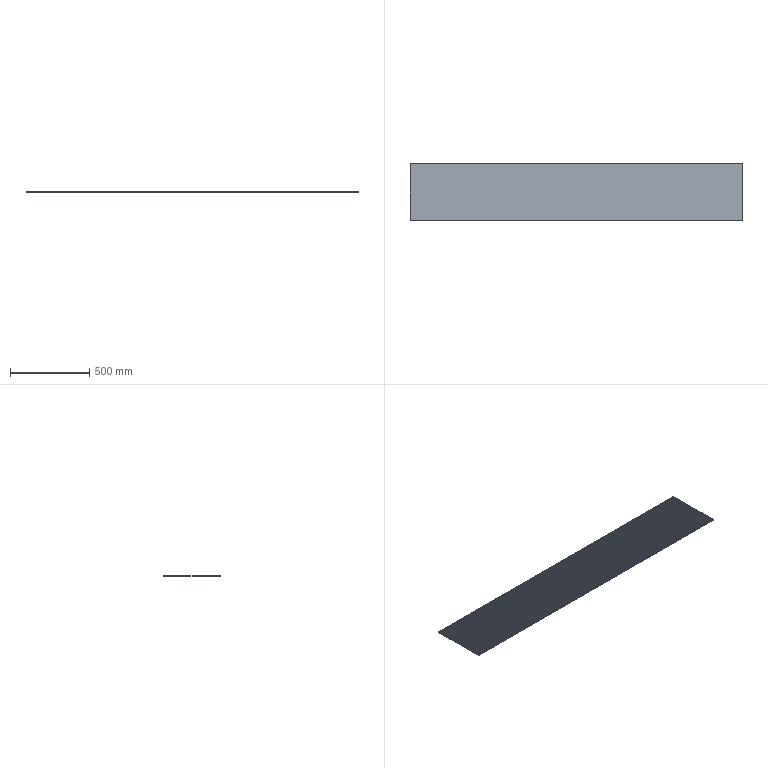Part | STEP file | 51E-01204JG10 | 1 solid | 1110 faces | box 2100 x 355 x 5 mm | volume 1842144 mm3 | cylinder 1104 | plane 6 | commonest cylinder face diameters 3.5 x1104